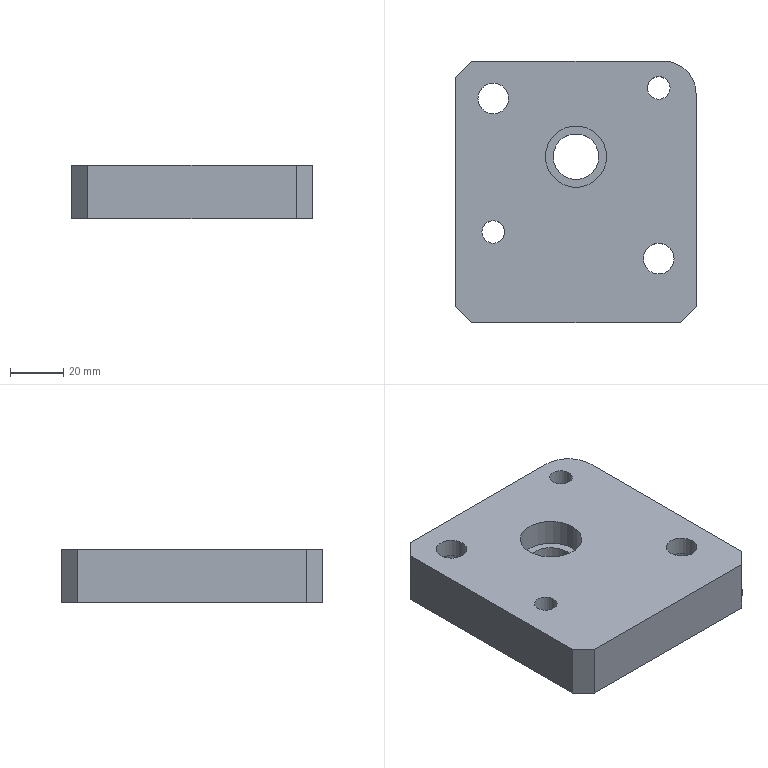Part | STEP file | lll_id3142_x_t | 1 solid | 21 faces | box 90 x 98 x 20 mm | volume 157900 mm3 | plane 12 | cylinder 9 | commonest cylinder face diameters 8.505 x2 11.509 x2 18.007 x2 17.1 x1 23 x1 24 x1
STEP:
#1=CARTESIAN_POINT('',(869.003,21.75,2.5));
#2=VERTEX_POINT('',#1);
#3=CARTESIAN_POINT('',(860.,21.75,2.5));
#4=DIRECTION('',(0.,0.,1.));
#5=DIRECTION('',(1.,0.,0.));
#6=AXIS2_PLACEMENT_3D('',#3,#4,#5);
#7=CIRCLE('',#6,9.004);
#8=EDGE_CURVE('',#2,#2,#7,.T.);
#9=ORIENTED_EDGE('',*,*,#8,.T.);
#10=EDGE_LOOP('',(#9));
#11=FACE_BOUND('',#10,.T.);
#12=CARTESIAN_POINT('',(917.747,25.75,2.5));
#13=VERTEX_POINT('',#12);
#14=CARTESIAN_POINT('',(922.,25.75,2.5));
#15=DIRECTION('',(0.,0.,-1.));
#16=DIRECTION('',(-1.,0.,0.));
#17=AXIS2_PLACEMENT_3D('',#14,#15,#16);
#18=CIRCLE('',#17,4.253);
#19=EDGE_CURVE('',#13,#13,#18,.T.);
#20=ORIENTED_EDGE('',*,*,#19,.F.);
#21=EDGE_LOOP('',(#20));
#22=FACE_BOUND('',#21,.T.);
#23=CARTESIAN_POINT('',(855.747,-28.25,2.5));
#24=VERTEX_POINT('',#23);
#25=CARTESIAN_POINT('',(860.,-28.25,2.5));
#26=DIRECTION('',(0.,0.,-1.));
#27=DIRECTION('',(-1.,0.,0.));
#28=AXIS2_PLACEMENT_3D('',#25,#26,#27);
#29=CIRCLE('',#28,4.253);
#30=EDGE_CURVE('',#24,#24,#29,.T.);
#31=ORIENTED_EDGE('',*,*,#30,.F.);
#32=EDGE_LOOP('',(#31));
#33=FACE_BOUND('',#32,.T.);
#34=CARTESIAN_POINT('',(924.,35.75,2.5));
#35=VERTEX_POINT('',#34);
#36=CARTESIAN_POINT('',(852.,35.75,2.5));
#37=VERTEX_POINT('',#36);
#38=CARTESIAN_POINT('',(891.,35.75,2.5));
#39=DIRECTION('',(-1.,0.,0.));
#40=VECTOR('',#39,1.);
#41=LINE('',#38,#40);
#42=EDGE_CURVE('',#35,#37,#41,.T.);
#43=ORIENTED_EDGE('',*,*,#42,.F.);
#44=CARTESIAN_POINT('',(936.,23.75,2.5));
#45=VERTEX_POINT('',#44);
#46=CARTESIAN_POINT('',(924.,23.75,2.5));
#47=DIRECTION('',(0.,0.,-1.));
#48=DIRECTION('',(-1.,0.,0.));
#49=AXIS2_PLACEMENT_3D('',#46,#47,#48);
#50=CIRCLE('',#49,12.);
#51=EDGE_CURVE('',#35,#45,#50,.T.);
#52=ORIENTED_EDGE('',*,*,#51,.T.);
#53=CARTESIAN_POINT('',(936.,-56.25,2.5));
#54=VERTEX_POINT('',#53);
#55=CARTESIAN_POINT('',(936.,-8.25,2.5));
#56=DIRECTION('',(0.,1.,0.));
#57=VECTOR('',#56,1.);
#58=LINE('',#55,#57);
#59=EDGE_CURVE('',#54,#45,#58,.T.);
#60=ORIENTED_EDGE('',*,*,#59,.F.);
#61=CARTESIAN_POINT('',(930.,-62.25,2.5));
#62=VERTEX_POINT('',#61);
#63=CARTESIAN_POINT('',(937.5,-54.75,2.5));
#64=DIRECTION('',(-0.7071,-0.7071,0.));
#65=VECTOR('',#64,1.);
#66=LINE('',#63,#65);
#67=EDGE_CURVE('',#54,#62,#66,.T.);
#68=ORIENTED_EDGE('',*,*,#67,.T.);
#69=CARTESIAN_POINT('',(852.,-62.25,2.5));
#70=VERTEX_POINT('',#69);
#71=CARTESIAN_POINT('',(891.,-62.25,2.5));
#72=DIRECTION('',(1.,0.,0.));
#73=VECTOR('',#72,1.);
#74=LINE('',#71,#73);
#75=EDGE_CURVE('',#70,#62,#74,.T.);
#76=ORIENTED_EDGE('',*,*,#75,.F.);
#77=CARTESIAN_POINT('',(846.,-56.25,2.5));
#78=VERTEX_POINT('',#77);
#79=CARTESIAN_POINT('',(844.5,-54.75,2.5));
#80=DIRECTION('',(-0.7071,0.7071,0.));
#81=VECTOR('',#80,1.);
#82=LINE('',#79,#81);
#83=EDGE_CURVE('',#70,#78,#82,.T.);
#84=ORIENTED_EDGE('',*,*,#83,.T.);
#85=CARTESIAN_POINT('',(846.,29.75,2.5));
#86=VERTEX_POINT('',#85);
#87=CARTESIAN_POINT('',(846.,-8.25,2.5));
#88=DIRECTION('',(0.,-1.,0.));
#89=VECTOR('',#88,1.);
#90=LINE('',#87,#89);
#91=EDGE_CURVE('',#86,#78,#90,.T.);
#92=ORIENTED_EDGE('',*,*,#91,.F.);
#93=CARTESIAN_POINT('',(849.5,33.25,2.5));
#94=DIRECTION('',(0.7071,0.7071,0.));
#95=VECTOR('',#94,1.);
#96=LINE('',#93,#95);
#97=EDGE_CURVE('',#86,#37,#96,.T.);
#98=ORIENTED_EDGE('',*,*,#97,.T.);
#99=EDGE_LOOP('',(#43,#52,#60,#68,#76,#84,#92,#98));
#100=FACE_BOUND('',#99,.T.);
#101=CARTESIAN_POINT('',(882.45,0.,2.5));
#102=VERTEX_POINT('',#101);
#103=CARTESIAN_POINT('',(891.,0.,2.5));
#104=DIRECTION('',(0.,0.,1.));
#105=DIRECTION('',(-1.,0.,0.));
#106=AXIS2_PLACEMENT_3D('',#103,#104,#105);
#107=CIRCLE('',#106,8.55);
#108=EDGE_CURVE('',#102,#102,#107,.T.);
#109=ORIENTED_EDGE('',*,*,#108,.T.);
#110=EDGE_LOOP('',(#109));
#111=FACE_BOUND('',#110,.T.);
#112=CARTESIAN_POINT('',(931.003,-38.25,2.5));
#113=VERTEX_POINT('',#112);
#114=CARTESIAN_POINT('',(922.,-38.25,2.5));
#115=DIRECTION('',(0.,0.,1.));
#116=DIRECTION('',(1.,0.,0.));
#117=AXIS2_PLACEMENT_3D('',#114,#115,#116);
#118=CIRCLE('',#117,9.004);
#119=EDGE_CURVE('',#113,#113,#118,.T.);
#120=ORIENTED_EDGE('',*,*,#119,.T.);
#121=EDGE_LOOP('',(#120));
#122=FACE_BOUND('',#121,.T.);
#123=CARTESIAN_POINT('',(891.,-8.25,2.5));
#124=DIRECTION('',(0.,0.,-1.));
#125=DIRECTION('',(1.,0.,0.));
#126=AXIS2_PLACEMENT_3D('',#123,#124,#125);
#127=PLANE('',#126);
#128=ADVANCED_FACE('',(#11,#22,#33,#100,#111,#122),#127,.T.);
#129=CARTESIAN_POINT('',(927.754,-38.25,22.5));
#130=VERTEX_POINT('',#129);
#131=CARTESIAN_POINT('',(922.,-38.25,22.5));
#132=DIRECTION('',(0.,0.,1.));
#133=DIRECTION('',(1.,0.,0.));
#134=AXIS2_PLACEMENT_3D('',#131,#132,#133);
#135=CIRCLE('',#134,5.755);
#136=EDGE_CURVE('',#130,#130,#135,.T.);
#137=ORIENTED_EDGE('',*,*,#136,.F.);
#138=EDGE_LOOP('',(#137));
#139=FACE_BOUND('',#138,.T.);
#140=CARTESIAN_POINT('',(865.754,21.75,22.5));
#141=VERTEX_POINT('',#140);
#142=CARTESIAN_POINT('',(860.,21.75,22.5));
#143=DIRECTION('',(0.,0.,1.));
#144=DIRECTION('',(1.,0.,0.));
#145=AXIS2_PLACEMENT_3D('',#142,#143,#144);
#146=CIRCLE('',#145,5.755);
#147=EDGE_CURVE('',#141,#141,#146,.T.);
#148=ORIENTED_EDGE('',*,*,#147,.F.);
#149=EDGE_LOOP('',(#148));
#150=FACE_BOUND('',#149,.T.);
#151=CARTESIAN_POINT('',(926.252,25.75,22.5));
#152=VERTEX_POINT('',#151);
#153=CARTESIAN_POINT('',(922.,25.75,22.5));
#154=DIRECTION('',(0.,0.,1.));
#155=DIRECTION('',(1.,0.,0.));
#156=AXIS2_PLACEMENT_3D('',#153,#154,#155);
#157=CIRCLE('',#156,4.253);
#158=EDGE_CURVE('',#152,#152,#157,.T.);
#159=ORIENTED_EDGE('',*,*,#158,.F.);
#160=EDGE_LOOP('',(#159));
#161=FACE_BOUND('',#160,.T.);
#162=CARTESIAN_POINT('',(864.252,-28.25,22.5));
#163=VERTEX_POINT('',#162);
#164=CARTESIAN_POINT('',(860.,-28.25,22.5));
#165=DIRECTION('',(0.,0.,1.));
#166=DIRECTION('',(1.,0.,0.));
#167=AXIS2_PLACEMENT_3D('',#164,#165,#166);
#168=CIRCLE('',#167,4.253);
#169=EDGE_CURVE('',#163,#163,#168,.T.);
#170=ORIENTED_EDGE('',*,*,#169,.F.);
#171=EDGE_LOOP('',(#170));
#172=FACE_BOUND('',#171,.T.);
#173=CARTESIAN_POINT('',(936.,23.75,22.5));
#174=VERTEX_POINT('',#173);
#175=CARTESIAN_POINT('',(936.,-56.25,22.5));
#176=VERTEX_POINT('',#175);
#177=CARTESIAN_POINT('',(936.,-8.25,22.5));
#178=DIRECTION('',(0.,-1.,0.));
#179=VECTOR('',#178,1.);
#180=LINE('',#177,#179);
#181=EDGE_CURVE('',#174,#176,#180,.T.);
#182=ORIENTED_EDGE('',*,*,#181,.F.);
#183=CARTESIAN_POINT('',(924.,35.75,22.5));
#184=VERTEX_POINT('',#183);
#185=CARTESIAN_POINT('',(924.,23.75,22.5));
#186=DIRECTION('',(0.,0.,1.));
#187=DIRECTION('',(1.,0.,0.));
#188=AXIS2_PLACEMENT_3D('',#185,#186,#187);
#189=CIRCLE('',#188,12.);
#190=EDGE_CURVE('',#174,#184,#189,.T.);
#191=ORIENTED_EDGE('',*,*,#190,.T.);
#192=CARTESIAN_POINT('',(852.,35.75,22.5));
#193=VERTEX_POINT('',#192);
#194=CARTESIAN_POINT('',(891.,35.75,22.5));
#195=DIRECTION('',(1.,0.,0.));
#196=VECTOR('',#195,1.);
#197=LINE('',#194,#196);
#198=EDGE_CURVE('',#193,#184,#197,.T.);
#199=ORIENTED_EDGE('',*,*,#198,.F.);
#200=CARTESIAN_POINT('',(846.,29.75,22.5));
#201=VERTEX_POINT('',#200);
#202=CARTESIAN_POINT('',(849.5,33.25,22.5));
#203=DIRECTION('',(-0.7071,-0.7071,0.));
#204=VECTOR('',#203,1.);
#205=LINE('',#202,#204);
#206=EDGE_CURVE('',#193,#201,#205,.T.);
#207=ORIENTED_EDGE('',*,*,#206,.T.);
#208=CARTESIAN_POINT('',(846.,-56.25,22.5));
#209=VERTEX_POINT('',#208);
#210=CARTESIAN_POINT('',(846.,-8.25,22.5));
#211=DIRECTION('',(0.,1.,0.));
#212=VECTOR('',#211,1.);
#213=LINE('',#210,#212);
#214=EDGE_CURVE('',#209,#201,#213,.T.);
#215=ORIENTED_EDGE('',*,*,#214,.F.);
#216=CARTESIAN_POINT('',(852.,-62.25,22.5));
#217=VERTEX_POINT('',#216);
#218=CARTESIAN_POINT('',(844.5,-54.75,22.5));
#219=DIRECTION('',(0.7071,-0.7071,0.));
#220=VECTOR('',#219,1.);
#221=LINE('',#218,#220);
#222=EDGE_CURVE('',#209,#217,#221,.T.);
#223=ORIENTED_EDGE('',*,*,#222,.T.);
#224=CARTESIAN_POINT('',(930.,-62.25,22.5));
#225=VERTEX_POINT('',#224);
#226=CARTESIAN_POINT('',(891.,-62.25,22.5));
#227=DIRECTION('',(-1.,0.,0.));
#228=VECTOR('',#227,1.);
#229=LINE('',#226,#228);
#230=EDGE_CURVE('',#225,#217,#229,.T.);
#231=ORIENTED_EDGE('',*,*,#230,.F.);
#232=CARTESIAN_POINT('',(937.5,-54.75,22.5));
#233=DIRECTION('',(0.7071,0.7071,0.));
#234=VECTOR('',#233,1.);
#235=LINE('',#232,#234);
#236=EDGE_CURVE('',#225,#176,#235,.T.);
#237=ORIENTED_EDGE('',*,*,#236,.T.);
#238=EDGE_LOOP('',(#182,#191,#199,#207,#215,#223,#231,#237));
#239=FACE_BOUND('',#238,.T.);
#240=CARTESIAN_POINT('',(902.5,0.,22.5));
#241=VERTEX_POINT('',#240);
#242=CARTESIAN_POINT('',(891.,0.,22.5));
#243=DIRECTION('',(0.,0.,-1.));
#244=DIRECTION('',(1.,0.,0.));
#245=AXIS2_PLACEMENT_3D('',#242,#243,#244);
#246=CIRCLE('',#245,11.5);
#247=EDGE_CURVE('',#241,#241,#246,.T.);
#248=ORIENTED_EDGE('',*,*,#247,.T.);
#249=EDGE_LOOP('',(#248));
#250=FACE_BOUND('',#249,.T.);
#251=CARTESIAN_POINT('',(891.,-8.25,22.5));
#252=DIRECTION('',(0.,0.,1.));
#253=DIRECTION('',(-1.,0.,0.));
#254=AXIS2_PLACEMENT_3D('',#251,#252,#253);
#255=PLANE('',#254);
#256=ADVANCED_FACE('',(#139,#150,#161,#172,#239,#250),#255,.T.);
#257=ORIENTED_EDGE('',*,*,#198,.T.);
#258=CARTESIAN_POINT('',(924.,35.75,2.5));
#259=DIRECTION('',(0.,0.,-1.));
#260=VECTOR('',#259,1.);
#261=LINE('',#258,#260);
#262=EDGE_CURVE('',#184,#35,#261,.T.);
#263=ORIENTED_EDGE('',*,*,#262,.T.);
#264=ORIENTED_EDGE('',*,*,#42,.T.);
#265=CARTESIAN_POINT('',(852.,35.75,2.5));
#266=DIRECTION('',(0.,0.,1.));
#267=VECTOR('',#266,1.);
#268=LINE('',#265,#267);
#269=EDGE_CURVE('',#37,#193,#268,.T.);
#270=ORIENTED_EDGE('',*,*,#269,.T.);
#271=EDGE_LOOP('',(#257,#263,#264,#270));
#272=FACE_OUTER_BOUND('',#271,.T.);
#273=CARTESIAN_POINT('',(891.,35.75,2.5));
#274=DIRECTION('',(0.,1.,0.));
#275=DIRECTION('',(0.,0.,-1.));
#276=AXIS2_PLACEMENT_3D('',#273,#274,#275);
#277=PLANE('',#276);
#278=ADVANCED_FACE('',(#272),#277,.T.);
#279=ORIENTED_EDGE('',*,*,#59,.T.);
#280=CARTESIAN_POINT('',(936.,23.75,2.5));
#281=DIRECTION('',(0.,0.,1.));
#282=VECTOR('',#281,1.);
#283=LINE('',#280,#282);
#284=EDGE_CURVE('',#45,#174,#283,.T.);
#285=ORIENTED_EDGE('',*,*,#284,.T.);
#286=ORIENTED_EDGE('',*,*,#181,.T.);
#287=CARTESIAN_POINT('',(936.,-56.25,2.5));
#288=DIRECTION('',(0.,0.,-1.));
#289=VECTOR('',#288,1.);
#290=LINE('',#287,#289);
#291=EDGE_CURVE('',#176,#54,#290,.T.);
#292=ORIENTED_EDGE('',*,*,#291,.T.);
#293=EDGE_LOOP('',(#279,#285,#286,#292));
#294=FACE_OUTER_BOUND('',#293,.T.);
#295=CARTESIAN_POINT('',(936.,-8.25,2.5));
#296=DIRECTION('',(1.,0.,0.));
#297=DIRECTION('',(0.,0.,1.));
#298=AXIS2_PLACEMENT_3D('',#295,#296,#297);
#299=PLANE('',#298);
#300=ADVANCED_FACE('',(#294),#299,.T.);
#301=ORIENTED_EDGE('',*,*,#230,.T.);
#302=CARTESIAN_POINT('',(852.,-62.25,2.5));
#303=DIRECTION('',(0.,0.,-1.));
#304=VECTOR('',#303,1.);
#305=LINE('',#302,#304);
#306=EDGE_CURVE('',#217,#70,#305,.T.);
#307=ORIENTED_EDGE('',*,*,#306,.T.);
#308=ORIENTED_EDGE('',*,*,#75,.T.);
#309=CARTESIAN_POINT('',(930.,-62.25,2.5));
#310=DIRECTION('',(0.,0.,1.));
#311=VECTOR('',#310,1.);
#312=LINE('',#309,#311);
#313=EDGE_CURVE('',#62,#225,#312,.T.);
#314=ORIENTED_EDGE('',*,*,#313,.T.);
#315=EDGE_LOOP('',(#301,#307,#308,#314));
#316=FACE_OUTER_BOUND('',#315,.T.);
#317=CARTESIAN_POINT('',(891.,-62.25,2.5));
#318=DIRECTION('',(0.,-1.,0.));
#319=DIRECTION('',(0.,0.,1.));
#320=AXIS2_PLACEMENT_3D('',#317,#318,#319);
#321=PLANE('',#320);
#322=ADVANCED_FACE('',(#316),#321,.T.);
#323=ORIENTED_EDGE('',*,*,#91,.T.);
#324=CARTESIAN_POINT('',(846.,-56.25,2.5));
#325=DIRECTION('',(0.,0.,1.));
#326=VECTOR('',#325,1.);
#327=LINE('',#324,#326);
#328=EDGE_CURVE('',#78,#209,#327,.T.);
#329=ORIENTED_EDGE('',*,*,#328,.T.);
#330=ORIENTED_EDGE('',*,*,#214,.T.);
#331=CARTESIAN_POINT('',(846.,29.75,2.5));
#332=DIRECTION('',(0.,0.,-1.));
#333=VECTOR('',#332,1.);
#334=LINE('',#331,#333);
#335=EDGE_CURVE('',#201,#86,#334,.T.);
#336=ORIENTED_EDGE('',*,*,#335,.T.);
#337=EDGE_LOOP('',(#323,#329,#330,#336));
#338=FACE_OUTER_BOUND('',#337,.T.);
#339=CARTESIAN_POINT('',(846.,-8.25,2.5));
#340=DIRECTION('',(-1.,0.,0.));
#341=DIRECTION('',(0.,0.,-1.));
#342=AXIS2_PLACEMENT_3D('',#339,#340,#341);
#343=PLANE('',#342);
#344=ADVANCED_FACE('',(#338),#343,.T.);
#345=CARTESIAN_POINT('',(882.45,0.,12.5));
#346=VERTEX_POINT('',#345);
#347=CARTESIAN_POINT('',(891.,0.,12.5));
#348=DIRECTION('',(0.,0.,-1.));
#349=DIRECTION('',(-1.,0.,0.));
#350=AXIS2_PLACEMENT_3D('',#347,#348,#349);
#351=CIRCLE('',#350,8.55);
#352=EDGE_CURVE('',#346,#346,#351,.T.);
#353=ORIENTED_EDGE('',*,*,#352,.F.);
#354=EDGE_LOOP('',(#353));
#355=FACE_BOUND('',#354,.T.);
#356=ORIENTED_EDGE('',*,*,#108,.F.);
#357=EDGE_LOOP('',(#356));
#358=FACE_BOUND('',#357,.T.);
#359=CARTESIAN_POINT('',(891.,0.,125.));
#360=DIRECTION('',(0.,0.,-1.));
#361=DIRECTION('',(1.,0.,0.));
#362=AXIS2_PLACEMENT_3D('',#359,#360,#361);
#363=CYLINDRICAL_SURFACE('',#362,8.55);
#364=ADVANCED_FACE('',(#355,#358),#363,.F.);
#365=CARTESIAN_POINT('',(879.5,0.,12.5));
#366=VERTEX_POINT('',#365);
#367=CARTESIAN_POINT('',(891.,0.,12.5));
#368=DIRECTION('',(0.,0.,1.));
#369=DIRECTION('',(-1.,0.,0.));
#370=AXIS2_PLACEMENT_3D('',#367,#368,#369);
#371=CIRCLE('',#370,11.5);
#372=EDGE_CURVE('',#366,#366,#371,.T.);
#373=ORIENTED_EDGE('',*,*,#372,.F.);
#374=EDGE_LOOP('',(#373));
#375=FACE_BOUND('',#374,.T.);
#376=ORIENTED_EDGE('',*,*,#247,.F.);
#377=EDGE_LOOP('',(#376));
#378=FACE_BOUND('',#377,.T.);
#379=CARTESIAN_POINT('',(891.,0.,12.5));
#380=DIRECTION('',(0.,0.,1.));
#381=DIRECTION('',(1.,0.,0.));
#382=AXIS2_PLACEMENT_3D('',#379,#380,#381);
#383=CYLINDRICAL_SURFACE('',#382,11.5);
#384=ADVANCED_FACE('',(#375,#378),#383,.F.);
#385=ORIENTED_EDGE('',*,*,#352,.T.);
#386=EDGE_LOOP('',(#385));
#387=FACE_BOUND('',#386,.T.);
#388=ORIENTED_EDGE('',*,*,#372,.T.);
#389=EDGE_LOOP('',(#388));
#390=FACE_BOUND('',#389,.T.);
#391=CARTESIAN_POINT('',(891.,0.,12.5));
#392=DIRECTION('',(0.,0.,-1.));
#393=DIRECTION('',(-1.,0.,0.));
#394=AXIS2_PLACEMENT_3D('',#391,#392,#393);
#395=PLANE('',#394);
#396=ADVANCED_FACE('',(#387,#390),#395,.F.);
#397=ORIENTED_EDGE('',*,*,#169,.T.);
#398=EDGE_LOOP('',(#397));
#399=FACE_BOUND('',#398,.T.);
#400=ORIENTED_EDGE('',*,*,#30,.T.);
#401=EDGE_LOOP('',(#400));
#402=FACE_BOUND('',#401,.T.);
#403=CARTESIAN_POINT('',(860.,-28.25,-2.5));
#404=DIRECTION('',(0.,0.,1.));
#405=DIRECTION('',(1.,0.,0.));
#406=AXIS2_PLACEMENT_3D('',#403,#404,#405);
#407=CYLINDRICAL_SURFACE('',#406,4.253);
#408=ADVANCED_FACE('',(#399,#402),#407,.F.);
#409=ORIENTED_EDGE('',*,*,#158,.T.);
#410=EDGE_LOOP('',(#409));
#411=FACE_BOUND('',#410,.T.);
#412=ORIENTED_EDGE('',*,*,#19,.T.);
#413=EDGE_LOOP('',(#412));
#414=FACE_BOUND('',#413,.T.);
#415=CARTESIAN_POINT('',(922.,25.75,-2.5));
#416=DIRECTION('',(0.,0.,1.));
#417=DIRECTION('',(1.,0.,0.));
#418=AXIS2_PLACEMENT_3D('',#415,#416,#417);
#419=CYLINDRICAL_SURFACE('',#418,4.253);
#420=ADVANCED_FACE('',(#411,#414),#419,.F.);
#421=ORIENTED_EDGE('',*,*,#147,.T.);
#422=EDGE_LOOP('',(#421));
#423=FACE_BOUND('',#422,.T.);
#424=CARTESIAN_POINT('',(865.754,21.75,15.5));
#425=VERTEX_POINT('',#424);
#426=CARTESIAN_POINT('',(860.,21.75,15.5));
#427=DIRECTION('',(0.,0.,1.));
#428=DIRECTION('',(1.,0.,0.));
#429=AXIS2_PLACEMENT_3D('',#426,#427,#428);
#430=CIRCLE('',#429,5.755);
#431=EDGE_CURVE('',#425,#425,#430,.T.);
#432=ORIENTED_EDGE('',*,*,#431,.F.);
#433=EDGE_LOOP('',(#432));
#434=FACE_BOUND('',#433,.T.);
#435=CARTESIAN_POINT('',(860.,21.75,-2.5));
#436=DIRECTION('',(0.,0.,1.));
#437=DIRECTION('',(1.,0.,0.));
#438=AXIS2_PLACEMENT_3D('',#435,#436,#437);
#439=CYLINDRICAL_SURFACE('',#438,5.755);
#440=ADVANCED_FACE('',(#423,#434),#439,.F.);
#441=ORIENTED_EDGE('',*,*,#431,.T.);
#442=EDGE_LOOP('',(#441));
#443=FACE_BOUND('',#442,.T.);
#444=CARTESIAN_POINT('',(869.003,21.75,15.5));
#445=VERTEX_POINT('',#444);
#446=CARTESIAN_POINT('',(860.,21.75,15.5));
#447=DIRECTION('',(0.,0.,1.));
#448=DIRECTION('',(1.,0.,0.));
#449=AXIS2_PLACEMENT_3D('',#446,#447,#448);
#450=CIRCLE('',#449,9.004);
#451=EDGE_CURVE('',#445,#445,#450,.T.);
#452=ORIENTED_EDGE('',*,*,#451,.F.);
#453=EDGE_LOOP('',(#452));
#454=FACE_BOUND('',#453,.T.);
#455=CARTESIAN_POINT('',(860.,21.75,15.5));
#456=DIRECTION('',(0.,0.,1.));
#457=DIRECTION('',(1.,0.,0.));
#458=AXIS2_PLACEMENT_3D('',#455,#456,#457);
#459=PLANE('',#458);
#460=ADVANCED_FACE('',(#443,#454),#459,.F.);
#461=ORIENTED_EDGE('',*,*,#451,.T.);
#462=EDGE_LOOP('',(#461));
#463=FACE_BOUND('',#462,.T.);
#464=ORIENTED_EDGE('',*,*,#8,.F.);
#465=EDGE_LOOP('',(#464));
#466=FACE_BOUND('',#465,.T.);
#467=CARTESIAN_POINT('',(860.,21.75,2.5));
#468=DIRECTION('',(0.,0.,1.));
#469=DIRECTION('',(1.,0.,0.));
#470=AXIS2_PLACEMENT_3D('',#467,#468,#469);
#471=CYLINDRICAL_SURFACE('',#470,9.004);
#472=ADVANCED_FACE('',(#463,#466),#471,.F.);
#473=ORIENTED_EDGE('',*,*,#136,.T.);
#474=EDGE_LOOP('',(#473));
#475=FACE_BOUND('',#474,.T.);
#476=CARTESIAN_POINT('',(927.754,-38.25,15.5));
#477=VERTEX_POINT('',#476);
#478=CARTESIAN_POINT('',(922.,-38.25,15.5));
#479=DIRECTION('',(0.,0.,1.));
#480=DIRECTION('',(1.,0.,0.));
#481=AXIS2_PLACEMENT_3D('',#478,#479,#480);
#482=CIRCLE('',#481,5.755);
#483=EDGE_CURVE('',#477,#477,#482,.T.);
#484=ORIENTED_EDGE('',*,*,#483,.F.);
#485=EDGE_LOOP('',(#484));
#486=FACE_BOUND('',#485,.T.);
#487=CARTESIAN_POINT('',(922.,-38.25,-2.5));
#488=DIRECTION('',(0.,0.,1.));
#489=DIRECTION('',(1.,0.,0.));
#490=AXIS2_PLACEMENT_3D('',#487,#488,#489);
#491=CYLINDRICAL_SURFACE('',#490,5.755);
#492=ADVANCED_FACE('',(#475,#486),#491,.F.);
#493=ORIENTED_EDGE('',*,*,#483,.T.);
#494=EDGE_LOOP('',(#493));
#495=FACE_BOUND('',#494,.T.);
#496=CARTESIAN_POINT('',(931.003,-38.25,15.5));
#497=VERTEX_POINT('',#496);
#498=CARTESIAN_POINT('',(922.,-38.25,15.5));
#499=DIRECTION('',(0.,0.,1.));
#500=DIRECTION('',(1.,0.,0.));
#501=AXIS2_PLACEMENT_3D('',#498,#499,#500);
#502=CIRCLE('',#501,9.004);
#503=EDGE_CURVE('',#497,#497,#502,.T.);
#504=ORIENTED_EDGE('',*,*,#503,.F.);
#505=EDGE_LOOP('',(#504));
#506=FACE_BOUND('',#505,.T.);
#507=CARTESIAN_POINT('',(922.,-38.25,15.5));
#508=DIRECTION('',(0.,0.,1.));
#509=DIRECTION('',(1.,0.,0.));
#510=AXIS2_PLACEMENT_3D('',#507,#508,#509);
#511=PLANE('',#510);
#512=ADVANCED_FACE('',(#495,#506),#511,.F.);
#513=ORIENTED_EDGE('',*,*,#503,.T.);
#514=EDGE_LOOP('',(#513));
#515=FACE_BOUND('',#514,.T.);
#516=ORIENTED_EDGE('',*,*,#119,.F.);
#517=EDGE_LOOP('',(#516));
#518=FACE_BOUND('',#517,.T.);
#519=CARTESIAN_POINT('',(922.,-38.25,2.5));
#520=DIRECTION('',(0.,0.,1.));
#521=DIRECTION('',(1.,0.,0.));
#522=AXIS2_PLACEMENT_3D('',#519,#520,#521);
#523=CYLINDRICAL_SURFACE('',#522,9.004);
#524=ADVANCED_FACE('',(#515,#518),#523,.F.);
#525=ORIENTED_EDGE('',*,*,#83,.F.);
#526=ORIENTED_EDGE('',*,*,#306,.F.);
#527=ORIENTED_EDGE('',*,*,#222,.F.);
#528=ORIENTED_EDGE('',*,*,#328,.F.);
#529=EDGE_LOOP('',(#525,#526,#527,#528));
#530=FACE_OUTER_BOUND('',#529,.T.);
#531=CARTESIAN_POINT('',(846.,-56.25,2.5));
#532=DIRECTION('',(0.7071,0.7071,0.));
#533=DIRECTION('',(0.,0.,-1.));
#534=AXIS2_PLACEMENT_3D('',#531,#532,#533);
#535=PLANE('',#534);
#536=ADVANCED_FACE('',(#530),#535,.F.);
#537=ORIENTED_EDGE('',*,*,#67,.F.);
#538=ORIENTED_EDGE('',*,*,#291,.F.);
#539=ORIENTED_EDGE('',*,*,#236,.F.);
#540=ORIENTED_EDGE('',*,*,#313,.F.);
#541=EDGE_LOOP('',(#537,#538,#539,#540));
#542=FACE_OUTER_BOUND('',#541,.T.);
#543=CARTESIAN_POINT('',(930.,-62.25,2.5));
#544=DIRECTION('',(-0.7071,0.7071,0.));
#545=DIRECTION('',(0.,0.,-1.));
#546=AXIS2_PLACEMENT_3D('',#543,#544,#545);
#547=PLANE('',#546);
#548=ADVANCED_FACE('',(#542),#547,.F.);
#549=ORIENTED_EDGE('',*,*,#97,.F.);
#550=ORIENTED_EDGE('',*,*,#335,.F.);
#551=ORIENTED_EDGE('',*,*,#206,.F.);
#552=ORIENTED_EDGE('',*,*,#269,.F.);
#553=EDGE_LOOP('',(#549,#550,#551,#552));
#554=FACE_OUTER_BOUND('',#553,.T.);
#555=CARTESIAN_POINT('',(852.,35.75,2.5));
#556=DIRECTION('',(0.7071,-0.7071,0.));
#557=DIRECTION('',(0.,0.,-1.));
#558=AXIS2_PLACEMENT_3D('',#555,#556,#557);
#559=PLANE('',#558);
#560=ADVANCED_FACE('',(#554),#559,.F.);
#561=ORIENTED_EDGE('',*,*,#190,.F.);
#562=ORIENTED_EDGE('',*,*,#284,.F.);
#563=ORIENTED_EDGE('',*,*,#51,.F.);
#564=ORIENTED_EDGE('',*,*,#262,.F.);
#565=EDGE_LOOP('',(#561,#562,#563,#564));
#566=FACE_OUTER_BOUND('',#565,.T.);
#567=CARTESIAN_POINT('',(924.,23.75,2.5));
#568=DIRECTION('',(0.,0.,-1.));
#569=DIRECTION('',(1.,0.,0.));
#570=AXIS2_PLACEMENT_3D('',#567,#568,#569);
#571=CYLINDRICAL_SURFACE('',#570,12.);
#572=ADVANCED_FACE('',(#566),#571,.T.);
#573=CLOSED_SHELL('',(#128,#256,#278,#300,#322,#344,#364,#384,#396,#408,#420,#440,#460,#472,#492,#512,#524,#536,#548,#560,#572));
#574=MANIFOLD_SOLID_BREP('',#573);
#575=(LENGTH_UNIT()NAMED_UNIT(*)SI_UNIT(.MILLI.,.METRE.));
#576=UNCERTAINTY_MEASURE_WITH_UNIT(LENGTH_MEASURE(0.00002),#575,'','');
#577=(NAMED_UNIT(*)PLANE_ANGLE_UNIT()SI_UNIT($,.RADIAN.));
#578=PLANE_ANGLE_MEASURE_WITH_UNIT(PLANE_ANGLE_MEASURE(0.01745),#577);
#579=DIMENSIONAL_EXPONENTS(0.,0.,0.,0.,0.,0.,0.);
#580=(CONVERSION_BASED_UNIT('DEGREE',#578)NAMED_UNIT(#579)PLANE_ANGLE_UNIT());
#581=(NAMED_UNIT(*)SI_UNIT($,.STERADIAN.)SOLID_ANGLE_UNIT());
#582=(GEOMETRIC_REPRESENTATION_CONTEXT(3)GLOBAL_UNCERTAINTY_ASSIGNED_CONTEXT((#576))GLOBAL_UNIT_ASSIGNED_CONTEXT((#575,#580,#581))REPRESENTATION_CONTEXT('',''));
#583=ADVANCED_BREP_SHAPE_REPRESENTATION('',(#574),#582);